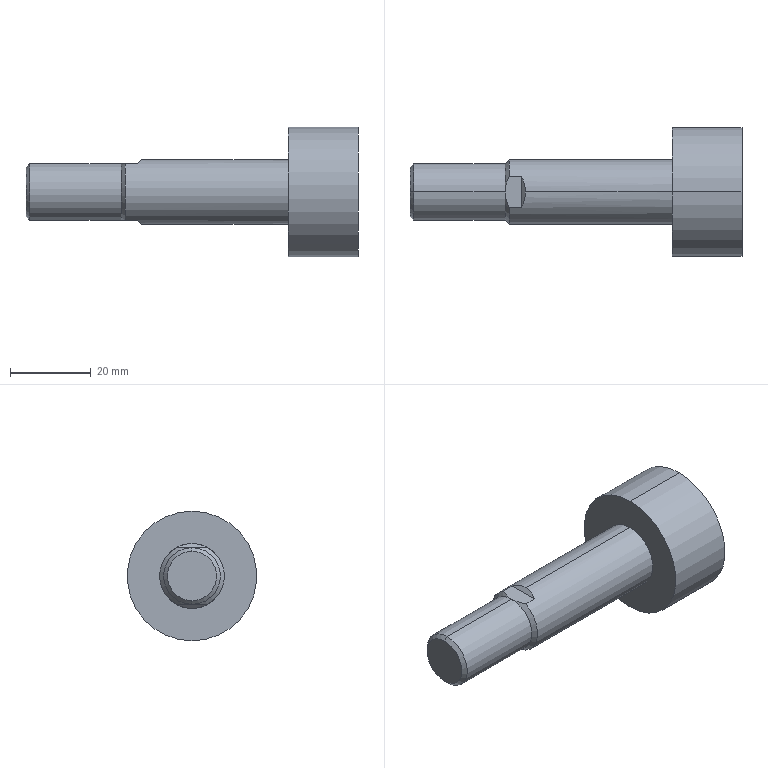Part | SolidWorks | features BaseBody 1 | 1 solid | 17 faces | box 82 x 32 x 32 mm | volume 25673 mm3 | plane 7 | cylinder 6 | cone 4 | commonest cylinder face diameters 14 x2 16 x2 32 x2
STEP:
#1=CARTESIAN_POINT('',(36.3,0.,8.));
#2=VERTEX_POINT('',#1);
#3=CARTESIAN_POINT('',(36.3,0.,-8.));
#4=VERTEX_POINT('',#3);
#5=CARTESIAN_POINT('',(36.3,0.,0.));
#6=DIRECTION('',(1.,0.,0.));
#7=DIRECTION('',(0.,0.,-1.));
#8=AXIS2_PLACEMENT_3D('',#5,#6,#7);
#9=CIRCLE('',#8,8.);
#10=EDGE_CURVE('',#2,#4,#9,.T.);
#11=ORIENTED_EDGE('',*,*,#10,.F.);
#12=CARTESIAN_POINT('',(0.,0.,8.));
#13=VERTEX_POINT('',#12);
#14=CARTESIAN_POINT('',(53.5,0.,8.));
#15=DIRECTION('',(-1.,0.,0.));
#16=VECTOR('',#15,1000.);
#17=LINE('',#14,#16);
#18=EDGE_CURVE('',#2,#13,#17,.T.);
#19=ORIENTED_EDGE('',*,*,#18,.T.);
#20=CARTESIAN_POINT('',(-1.,-3.873,7.));
#21=VERTEX_POINT('',#20);
#22=CARTESIAN_POINT('',(-1.,-3.873,7.));
#23=CARTESIAN_POINT('',(-0.3405,-2.681,7.659));
#24=CARTESIAN_POINT('',(0.,-1.362,8.));
#25=CARTESIAN_POINT('',(0.,0.,8.));
#26=(BOUNDED_CURVE()B_SPLINE_CURVE(3,(#22,#23,#24,#25),.UNSPECIFIED.,.F.,.F.)B_SPLINE_CURVE_WITH_KNOTS((4,4),(5.778,6.283),.UNSPECIFIED.)CURVE()GEOMETRIC_REPRESENTATION_ITEM()RATIONAL_B_SPLINE_CURVE((1.,0.9788,0.9788,1.))REPRESENTATION_ITEM(''));
#27=EDGE_CURVE('',#21,#13,#26,.T.);
#28=ORIENTED_EDGE('',*,*,#27,.F.);
#29=CARTESIAN_POINT('',(-4.,-3.873,7.));
#30=VERTEX_POINT('',#29);
#31=CARTESIAN_POINT('',(53.5,-3.873,7.));
#32=DIRECTION('',(1.,0.,0.));
#33=VECTOR('',#32,1000.);
#34=LINE('',#31,#33);
#35=EDGE_CURVE('',#30,#21,#34,.T.);
#36=ORIENTED_EDGE('',*,*,#35,.F.);
#37=CARTESIAN_POINT('',(-4.,-3.873,-7.));
#38=VERTEX_POINT('',#37);
#39=CARTESIAN_POINT('',(-4.,0.,0.));
#40=DIRECTION('',(1.,0.,0.));
#41=DIRECTION('',(0.,0.,-1.));
#42=AXIS2_PLACEMENT_3D('',#39,#40,#41);
#43=CIRCLE('',#42,8.);
#44=EDGE_CURVE('',#30,#38,#43,.T.);
#45=ORIENTED_EDGE('',*,*,#44,.T.);
#46=CARTESIAN_POINT('',(-1.,-3.873,-7.));
#47=VERTEX_POINT('',#46);
#48=CARTESIAN_POINT('',(53.5,-3.873,-7.));
#49=DIRECTION('',(-1.,0.,0.));
#50=VECTOR('',#49,1000.);
#51=LINE('',#48,#50);
#52=EDGE_CURVE('',#47,#38,#51,.T.);
#53=ORIENTED_EDGE('',*,*,#52,.F.);
#54=CARTESIAN_POINT('',(0.,0.,-8.));
#55=VERTEX_POINT('',#54);
#56=CARTESIAN_POINT('',(0.,0.,-8.));
#57=CARTESIAN_POINT('',(0.,-1.362,-8.));
#58=CARTESIAN_POINT('',(-0.3405,-2.681,-7.659));
#59=CARTESIAN_POINT('',(-1.,-3.873,-7.));
#60=(BOUNDED_CURVE()B_SPLINE_CURVE(3,(#56,#57,#58,#59),.UNSPECIFIED.,.F.,.F.)B_SPLINE_CURVE_WITH_KNOTS((4,4),(0.,0.5054),.UNSPECIFIED.)CURVE()GEOMETRIC_REPRESENTATION_ITEM()RATIONAL_B_SPLINE_CURVE((1.,0.9788,0.9788,1.))REPRESENTATION_ITEM(''));
#61=EDGE_CURVE('',#55,#47,#60,.T.);
#62=ORIENTED_EDGE('',*,*,#61,.F.);
#63=CARTESIAN_POINT('',(53.5,0.,-8.));
#64=DIRECTION('',(-1.,0.,0.));
#65=VECTOR('',#64,1000.);
#66=LINE('',#63,#65);
#67=EDGE_CURVE('',#4,#55,#66,.T.);
#68=ORIENTED_EDGE('',*,*,#67,.F.);
#69=EDGE_LOOP('',(#11,#19,#28,#36,#45,#53,#62,#68));
#70=FACE_OUTER_BOUND('',#69,.T.);
#71=CARTESIAN_POINT('',(53.5,0.,0.));
#72=DIRECTION('',(-1.,0.,0.));
#73=DIRECTION('',(0.,0.,-1.));
#74=AXIS2_PLACEMENT_3D('',#71,#72,#73);
#75=CYLINDRICAL_SURFACE('',#74,8.);
#76=ADVANCED_FACE('',(#70),#75,.T.);
#77=CARTESIAN_POINT('',(-5.,0.,7.));
#78=VERTEX_POINT('',#77);
#79=CARTESIAN_POINT('',(-5.,0.,-7.));
#80=VERTEX_POINT('',#79);
#81=CARTESIAN_POINT('',(-5.,0.,0.));
#82=DIRECTION('',(1.,0.,0.));
#83=DIRECTION('',(0.,0.,-1.));
#84=AXIS2_PLACEMENT_3D('',#81,#82,#83);
#85=CIRCLE('',#84,7.);
#86=EDGE_CURVE('',#78,#80,#85,.T.);
#87=ORIENTED_EDGE('',*,*,#86,.F.);
#88=CARTESIAN_POINT('',(-27.58,0.,7.));
#89=VERTEX_POINT('',#88);
#90=CARTESIAN_POINT('',(0.,0.,7.));
#91=DIRECTION('',(-1.,0.,0.));
#92=VECTOR('',#91,1000.);
#93=LINE('',#90,#92);
#94=EDGE_CURVE('',#78,#89,#93,.T.);
#95=ORIENTED_EDGE('',*,*,#94,.T.);
#96=CARTESIAN_POINT('',(-27.58,0.,-7.));
#97=VERTEX_POINT('',#96);
#98=CARTESIAN_POINT('',(-27.58,0.,0.));
#99=DIRECTION('',(1.,0.,0.));
#100=DIRECTION('',(0.,0.,-1.));
#101=AXIS2_PLACEMENT_3D('',#98,#99,#100);
#102=CIRCLE('',#101,7.);
#103=EDGE_CURVE('',#89,#97,#102,.T.);
#104=ORIENTED_EDGE('',*,*,#103,.T.);
#105=CARTESIAN_POINT('',(0.,0.,-7.));
#106=DIRECTION('',(-1.,0.,0.));
#107=VECTOR('',#106,1000.);
#108=LINE('',#105,#107);
#109=EDGE_CURVE('',#80,#97,#108,.T.);
#110=ORIENTED_EDGE('',*,*,#109,.F.);
#111=EDGE_LOOP('',(#87,#95,#104,#110));
#112=FACE_OUTER_BOUND('',#111,.T.);
#113=CARTESIAN_POINT('',(0.,0.,0.));
#114=DIRECTION('',(-1.,0.,0.));
#115=DIRECTION('',(0.,0.,-1.));
#116=AXIS2_PLACEMENT_3D('',#113,#114,#115);
#117=CYLINDRICAL_SURFACE('',#116,7.);
#118=ADVANCED_FACE('',(#112),#117,.T.);
#119=CARTESIAN_POINT('',(-28.5,0.,-6.08));
#120=VERTEX_POINT('',#119);
#121=CARTESIAN_POINT('',(-28.5,0.,6.08));
#122=VERTEX_POINT('',#121);
#123=CARTESIAN_POINT('',(-28.5,0.,0.));
#124=DIRECTION('',(1.,0.,0.));
#125=DIRECTION('',(0.,0.,-1.));
#126=AXIS2_PLACEMENT_3D('',#123,#124,#125);
#127=CIRCLE('',#126,6.08);
#128=EDGE_CURVE('',#120,#122,#127,.T.);
#129=ORIENTED_EDGE('',*,*,#128,.T.);
#130=CARTESIAN_POINT('',(-28.5,0.,6.08));
#131=DIRECTION('',(0.7071,0.,0.7071));
#132=VECTOR('',#131,1000.);
#133=LINE('',#130,#132);
#134=EDGE_CURVE('',#122,#89,#133,.T.);
#135=ORIENTED_EDGE('',*,*,#134,.T.);
#136=CARTESIAN_POINT('',(-27.58,0.,0.));
#137=DIRECTION('',(1.,0.,0.));
#138=DIRECTION('',(0.,0.,-1.));
#139=AXIS2_PLACEMENT_3D('',#136,#137,#138);
#140=CIRCLE('',#139,7.);
#141=EDGE_CURVE('',#97,#89,#140,.T.);
#142=ORIENTED_EDGE('',*,*,#141,.F.);
#143=CARTESIAN_POINT('',(-28.5,0.,-6.08));
#144=DIRECTION('',(0.7071,0.,-0.7071));
#145=VECTOR('',#144,1000.);
#146=LINE('',#143,#145);
#147=EDGE_CURVE('',#120,#97,#146,.T.);
#148=ORIENTED_EDGE('',*,*,#147,.F.);
#149=EDGE_LOOP('',(#129,#135,#142,#148));
#150=FACE_OUTER_BOUND('',#149,.T.);
#151=CARTESIAN_POINT('',(-28.5,0.,0.));
#152=DIRECTION('',(1.,0.,0.));
#153=DIRECTION('',(0.,0.,-1.));
#154=AXIS2_PLACEMENT_3D('',#151,#152,#153);
#155=CONICAL_SURFACE('',#154,6.08,0.7854);
#156=ADVANCED_FACE('',(#150),#155,.T.);
#157=CARTESIAN_POINT('',(53.5,0.,16.));
#158=VERTEX_POINT('',#157);
#159=CARTESIAN_POINT('',(53.5,0.,-16.));
#160=VERTEX_POINT('',#159);
#161=CARTESIAN_POINT('',(53.5,0.,0.));
#162=DIRECTION('',(1.,0.,0.));
#163=DIRECTION('',(0.,0.,-1.));
#164=AXIS2_PLACEMENT_3D('',#161,#162,#163);
#165=CIRCLE('',#164,16.);
#166=EDGE_CURVE('',#158,#160,#165,.T.);
#167=ORIENTED_EDGE('',*,*,#166,.F.);
#168=CARTESIAN_POINT('',(36.3,0.,16.));
#169=VERTEX_POINT('',#168);
#170=CARTESIAN_POINT('',(53.5,0.,16.));
#171=DIRECTION('',(-1.,0.,0.));
#172=VECTOR('',#171,1000.);
#173=LINE('',#170,#172);
#174=EDGE_CURVE('',#158,#169,#173,.T.);
#175=ORIENTED_EDGE('',*,*,#174,.T.);
#176=CARTESIAN_POINT('',(36.3,0.,-16.));
#177=VERTEX_POINT('',#176);
#178=CARTESIAN_POINT('',(36.3,0.,0.));
#179=DIRECTION('',(1.,0.,0.));
#180=DIRECTION('',(0.,0.,-1.));
#181=AXIS2_PLACEMENT_3D('',#178,#179,#180);
#182=CIRCLE('',#181,16.);
#183=EDGE_CURVE('',#169,#177,#182,.T.);
#184=ORIENTED_EDGE('',*,*,#183,.T.);
#185=CARTESIAN_POINT('',(53.5,0.,-16.));
#186=DIRECTION('',(-1.,0.,0.));
#187=VECTOR('',#186,1000.);
#188=LINE('',#185,#187);
#189=EDGE_CURVE('',#160,#177,#188,.T.);
#190=ORIENTED_EDGE('',*,*,#189,.F.);
#191=EDGE_LOOP('',(#167,#175,#184,#190));
#192=FACE_OUTER_BOUND('',#191,.T.);
#193=CARTESIAN_POINT('',(53.5,0.,0.));
#194=DIRECTION('',(-1.,0.,0.));
#195=DIRECTION('',(0.,0.,-1.));
#196=AXIS2_PLACEMENT_3D('',#193,#194,#195);
#197=CYLINDRICAL_SURFACE('',#196,16.);
#198=ADVANCED_FACE('',(#192),#197,.T.);
#199=CARTESIAN_POINT('',(36.3,0.,0.));
#200=DIRECTION('',(1.,0.,0.));
#201=DIRECTION('',(0.,0.,-1.));
#202=AXIS2_PLACEMENT_3D('',#199,#200,#201);
#203=CIRCLE('',#202,8.);
#204=EDGE_CURVE('',#4,#2,#203,.T.);
#205=ORIENTED_EDGE('',*,*,#204,.T.);
#206=ORIENTED_EDGE('',*,*,#10,.T.);
#207=EDGE_LOOP('',(#205,#206));
#208=FACE_BOUND('',#207,.T.);
#209=CARTESIAN_POINT('',(36.3,0.,0.));
#210=DIRECTION('',(1.,0.,0.));
#211=DIRECTION('',(0.,0.,-1.));
#212=AXIS2_PLACEMENT_3D('',#209,#210,#211);
#213=CIRCLE('',#212,16.);
#214=EDGE_CURVE('',#177,#169,#213,.T.);
#215=ORIENTED_EDGE('',*,*,#214,.F.);
#216=ORIENTED_EDGE('',*,*,#183,.F.);
#217=EDGE_LOOP('',(#215,#216));
#218=FACE_OUTER_BOUND('',#217,.T.);
#219=CARTESIAN_POINT('',(36.3,8.,0.));
#220=DIRECTION('',(1.,0.,0.));
#221=DIRECTION('',(0.,1.,0.));
#222=AXIS2_PLACEMENT_3D('',#219,#220,#221);
#223=PLANE('',#222);
#224=ADVANCED_FACE('',(#208,#218),#223,.F.);
#225=ORIENTED_EDGE('',*,*,#174,.F.);
#226=CARTESIAN_POINT('',(53.5,0.,0.));
#227=DIRECTION('',(1.,0.,0.));
#228=DIRECTION('',(0.,0.,-1.));
#229=AXIS2_PLACEMENT_3D('',#226,#227,#228);
#230=CIRCLE('',#229,16.);
#231=EDGE_CURVE('',#160,#158,#230,.T.);
#232=ORIENTED_EDGE('',*,*,#231,.F.);
#233=ORIENTED_EDGE('',*,*,#189,.T.);
#234=ORIENTED_EDGE('',*,*,#214,.T.);
#235=EDGE_LOOP('',(#225,#232,#233,#234));
#236=FACE_OUTER_BOUND('',#235,.T.);
#237=CARTESIAN_POINT('',(53.5,0.,0.));
#238=DIRECTION('',(-1.,0.,0.));
#239=DIRECTION('',(0.,0.,-1.));
#240=AXIS2_PLACEMENT_3D('',#237,#238,#239);
#241=CYLINDRICAL_SURFACE('',#240,16.);
#242=ADVANCED_FACE('',(#236),#241,.T.);
#243=ORIENTED_EDGE('',*,*,#231,.T.);
#244=ORIENTED_EDGE('',*,*,#166,.T.);
#245=EDGE_LOOP('',(#243,#244));
#246=FACE_OUTER_BOUND('',#245,.T.);
#247=CARTESIAN_POINT('',(53.5,16.,0.));
#248=DIRECTION('',(-1.,0.,0.));
#249=DIRECTION('',(0.,0.,1.));
#250=AXIS2_PLACEMENT_3D('',#247,#248,#249);
#251=PLANE('',#250);
#252=ADVANCED_FACE('',(#246),#251,.F.);
#253=ORIENTED_EDGE('',*,*,#128,.F.);
#254=CARTESIAN_POINT('',(-28.5,0.,0.));
#255=DIRECTION('',(1.,0.,0.));
#256=DIRECTION('',(0.,0.,-1.));
#257=AXIS2_PLACEMENT_3D('',#254,#255,#256);
#258=CIRCLE('',#257,6.08);
#259=EDGE_CURVE('',#122,#120,#258,.T.);
#260=ORIENTED_EDGE('',*,*,#259,.F.);
#261=EDGE_LOOP('',(#253,#260));
#262=FACE_OUTER_BOUND('',#261,.T.);
#263=CARTESIAN_POINT('',(-28.5,0.,0.));
#264=DIRECTION('',(1.,0.,0.));
#265=DIRECTION('',(0.,1.,0.));
#266=AXIS2_PLACEMENT_3D('',#263,#264,#265);
#267=PLANE('',#266);
#268=ADVANCED_FACE('',(#262),#267,.F.);
#269=ORIENTED_EDGE('',*,*,#134,.F.);
#270=ORIENTED_EDGE('',*,*,#259,.T.);
#271=ORIENTED_EDGE('',*,*,#147,.T.);
#272=ORIENTED_EDGE('',*,*,#103,.F.);
#273=EDGE_LOOP('',(#269,#270,#271,#272));
#274=FACE_OUTER_BOUND('',#273,.T.);
#275=CARTESIAN_POINT('',(-28.5,0.,0.));
#276=DIRECTION('',(1.,0.,0.));
#277=DIRECTION('',(0.,0.,-1.));
#278=AXIS2_PLACEMENT_3D('',#275,#276,#277);
#279=CONICAL_SURFACE('',#278,6.08,0.7854);
#280=ADVANCED_FACE('',(#274),#279,.T.);
#281=ORIENTED_EDGE('',*,*,#94,.F.);
#282=CARTESIAN_POINT('',(-5.,0.,0.));
#283=DIRECTION('',(1.,0.,0.));
#284=DIRECTION('',(0.,0.,-1.));
#285=AXIS2_PLACEMENT_3D('',#282,#283,#284);
#286=CIRCLE('',#285,7.);
#287=EDGE_CURVE('',#80,#78,#286,.T.);
#288=ORIENTED_EDGE('',*,*,#287,.F.);
#289=ORIENTED_EDGE('',*,*,#109,.T.);
#290=ORIENTED_EDGE('',*,*,#141,.T.);
#291=EDGE_LOOP('',(#281,#288,#289,#290));
#292=FACE_OUTER_BOUND('',#291,.T.);
#293=CARTESIAN_POINT('',(0.,0.,0.));
#294=DIRECTION('',(-1.,0.,0.));
#295=DIRECTION('',(0.,0.,-1.));
#296=AXIS2_PLACEMENT_3D('',#293,#294,#295);
#297=CYLINDRICAL_SURFACE('',#296,7.);
#298=ADVANCED_FACE('',(#292),#297,.T.);
#299=ORIENTED_EDGE('',*,*,#27,.T.);
#300=CARTESIAN_POINT('',(-1.,3.873,7.));
#301=VERTEX_POINT('',#300);
#302=CARTESIAN_POINT('',(0.,0.,8.));
#303=CARTESIAN_POINT('',(0.,1.362,8.));
#304=CARTESIAN_POINT('',(-0.3405,2.681,7.659));
#305=CARTESIAN_POINT('',(-1.,3.873,7.));
#306=(BOUNDED_CURVE()B_SPLINE_CURVE(3,(#302,#303,#304,#305),.UNSPECIFIED.,.F.,.F.)B_SPLINE_CURVE_WITH_KNOTS((4,4),(0.,0.5054),.UNSPECIFIED.)CURVE()GEOMETRIC_REPRESENTATION_ITEM()RATIONAL_B_SPLINE_CURVE((1.,0.9788,0.9788,1.))REPRESENTATION_ITEM(''));
#307=EDGE_CURVE('',#13,#301,#306,.T.);
#308=ORIENTED_EDGE('',*,*,#307,.T.);
#309=CARTESIAN_POINT('',(-1.,14.,7.));
#310=DIRECTION('',(0.,-1.,0.));
#311=VECTOR('',#310,1000.);
#312=LINE('',#309,#311);
#313=EDGE_CURVE('',#301,#21,#312,.T.);
#314=ORIENTED_EDGE('',*,*,#313,.T.);
#315=EDGE_LOOP('',(#299,#308,#314));
#316=FACE_OUTER_BOUND('',#315,.T.);
#317=CARTESIAN_POINT('',(19.,14.,27.));
#318=DIRECTION('',(-0.7071,0.,0.7071));
#319=DIRECTION('',(0.,1.,0.));
#320=AXIS2_PLACEMENT_3D('',#317,#318,#319);
#321=PLANE('',#320);
#322=ADVANCED_FACE('',(#316),#321,.T.);
#323=CARTESIAN_POINT('',(-4.,3.873,-7.));
#324=VERTEX_POINT('',#323);
#325=CARTESIAN_POINT('',(-5.,0.,-7.));
#326=CARTESIAN_POINT('',(-5.,0.3255,-7.));
#327=CARTESIAN_POINT('',(-4.965,0.8186,-7.));
#328=CARTESIAN_POINT('',(-4.864,1.403,-7.));
#329=CARTESIAN_POINT('',(-4.798,1.697,-7.));
#330=CARTESIAN_POINT('',(-4.761,1.844,-7.));
#331=CARTESIAN_POINT('',(-4.742,1.918,-7.));
#332=CARTESIAN_POINT('',(-4.733,1.95,-7.));
#333=CARTESIAN_POINT('',(-4.728,1.971,-7.));
#334=CARTESIAN_POINT('',(-4.725,1.983,-7.));
#335=CARTESIAN_POINT('',(-4.559,2.589,-7.));
#336=CARTESIAN_POINT('',(-4.318,3.216,-7.));
#337=CARTESIAN_POINT('',(-4.,3.873,-7.));
#338=B_SPLINE_CURVE_WITH_KNOTS('',3,(#325,#326,#327,#328,#329,#330,#331,#332,#333,#334,#335,#336,#337),.UNSPECIFIED.,.F.,.F.,(4,1,1,1,1,1,2,2,4),(0.,0.25,0.375,0.4375,0.4687,0.4844,0.4922,0.5,1.),.UNSPECIFIED.);
#339=EDGE_CURVE('',#80,#324,#338,.T.);
#340=ORIENTED_EDGE('',*,*,#339,.F.);
#341=ORIENTED_EDGE('',*,*,#287,.T.);
#342=CARTESIAN_POINT('',(-4.,3.873,7.));
#343=VERTEX_POINT('',#342);
#344=CARTESIAN_POINT('',(-4.,3.873,7.));
#345=CARTESIAN_POINT('',(-4.159,3.545,7.));
#346=CARTESIAN_POINT('',(-4.368,3.064,7.));
#347=CARTESIAN_POINT('',(-4.562,2.521,7.));
#348=CARTESIAN_POINT('',(-4.646,2.255,7.));
#349=CARTESIAN_POINT('',(-4.685,2.123,7.));
#350=CARTESIAN_POINT('',(-4.704,2.058,7.));
#351=CARTESIAN_POINT('',(-4.712,2.03,7.));
#352=CARTESIAN_POINT('',(-4.717,2.011,7.));
#353=CARTESIAN_POINT('',(-4.719,2.003,7.));
#354=CARTESIAN_POINT('',(-4.907,1.315,7.));
#355=CARTESIAN_POINT('',(-5.,0.6513,7.));
#356=CARTESIAN_POINT('',(-5.,0.,7.));
#357=B_SPLINE_CURVE_WITH_KNOTS('',3,(#344,#345,#346,#347,#348,#349,#350,#351,#352,#353,#354,#355,#356),.UNSPECIFIED.,.F.,.F.,(4,1,1,1,1,1,2,2,4),(0.,0.25,0.375,0.4375,0.4688,0.4844,0.4922,0.5,1.),.UNSPECIFIED.);
#358=EDGE_CURVE('',#343,#78,#357,.T.);
#359=ORIENTED_EDGE('',*,*,#358,.F.);
#360=CARTESIAN_POINT('',(-4.,0.,0.));
#361=DIRECTION('',(1.,0.,0.));
#362=DIRECTION('',(0.,0.,-1.));
#363=AXIS2_PLACEMENT_3D('',#360,#361,#362);
#364=CIRCLE('',#363,8.);
#365=EDGE_CURVE('',#324,#343,#364,.T.);
#366=ORIENTED_EDGE('',*,*,#365,.F.);
#367=EDGE_LOOP('',(#340,#341,#359,#366));
#368=FACE_OUTER_BOUND('',#367,.T.);
#369=CARTESIAN_POINT('',(-5.,0.,0.));
#370=DIRECTION('',(1.,0.,0.));
#371=DIRECTION('',(0.,0.,-1.));
#372=AXIS2_PLACEMENT_3D('',#369,#370,#371);
#373=CONICAL_SURFACE('',#372,7.,0.7854);
#374=ADVANCED_FACE('',(#368),#373,.T.);
#375=CARTESIAN_POINT('',(-5.,0.,7.));
#376=CARTESIAN_POINT('',(-5.,-0.3269,7.));
#377=CARTESIAN_POINT('',(-4.965,-0.8222,7.));
#378=CARTESIAN_POINT('',(-4.863,-1.409,7.));
#379=CARTESIAN_POINT('',(-4.796,-1.704,7.));
#380=CARTESIAN_POINT('',(-4.759,-1.852,7.));
#381=CARTESIAN_POINT('',(-4.74,-1.927,7.));
#382=CARTESIAN_POINT('',(-4.731,-1.959,7.));
#383=CARTESIAN_POINT('',(-4.725,-1.98,7.));
#384=CARTESIAN_POINT('',(-4.722,-1.992,7.));
#385=CARTESIAN_POINT('',(-4.556,-2.595,7.));
#386=CARTESIAN_POINT('',(-4.316,-3.219,7.));
#387=CARTESIAN_POINT('',(-4.,-3.873,7.));
#388=B_SPLINE_CURVE_WITH_KNOTS('',3,(#375,#376,#377,#378,#379,#380,#381,#382,#383,#384,#385,#386,#387),.UNSPECIFIED.,.F.,.F.,(4,1,1,1,1,1,2,2,4),(0.,0.25,0.375,0.4375,0.4688,0.4844,0.4922,0.5,1.),.UNSPECIFIED.);
#389=EDGE_CURVE('',#78,#30,#388,.T.);
#390=ORIENTED_EDGE('',*,*,#389,.F.);
#391=ORIENTED_EDGE('',*,*,#86,.T.);
#392=CARTESIAN_POINT('',(-4.,-3.873,-7.));
#393=CARTESIAN_POINT('',(-4.158,-3.546,-7.));
#394=CARTESIAN_POINT('',(-4.367,-3.067,-7.));
#395=CARTESIAN_POINT('',(-4.56,-2.528,-7.));
#396=CARTESIAN_POINT('',(-4.644,-2.263,-7.));
#397=CARTESIAN_POINT('',(-4.683,-2.132,-7.));
#398=CARTESIAN_POINT('',(-4.701,-2.066,-7.));
#399=CARTESIAN_POINT('',(-4.709,-2.038,-7.));
#400=CARTESIAN_POINT('',(-4.714,-2.02,-7.));
#401=CARTESIAN_POINT('',(-4.717,-2.012,-7.));
#402=CARTESIAN_POINT('',(-4.907,-1.321,-7.));
#403=CARTESIAN_POINT('',(-5.,-0.6541,-7.));
#404=CARTESIAN_POINT('',(-5.,0.,-7.));
#405=B_SPLINE_CURVE_WITH_KNOTS('',3,(#392,#393,#394,#395,#396,#397,#398,#399,#400,#401,#402,#403,#404),.UNSPECIFIED.,.F.,.F.,(4,1,1,1,1,1,2,2,4),(0.,0.25,0.375,0.4375,0.4687,0.4844,0.4922,0.5,1.),.UNSPECIFIED.);
#406=EDGE_CURVE('',#38,#80,#405,.T.);
#407=ORIENTED_EDGE('',*,*,#406,.F.);
#408=ORIENTED_EDGE('',*,*,#44,.F.);
#409=EDGE_LOOP('',(#390,#391,#407,#408));
#410=FACE_OUTER_BOUND('',#409,.T.);
#411=CARTESIAN_POINT('',(-5.,0.,0.));
#412=DIRECTION('',(1.,0.,0.));
#413=DIRECTION('',(0.,0.,-1.));
#414=AXIS2_PLACEMENT_3D('',#411,#412,#413);
#415=CONICAL_SURFACE('',#414,7.,0.7854);
#416=ADVANCED_FACE('',(#410),#415,.T.);
#417=ORIENTED_EDGE('',*,*,#35,.T.);
#418=ORIENTED_EDGE('',*,*,#313,.F.);
#419=CARTESIAN_POINT('',(53.5,3.873,7.));
#420=DIRECTION('',(-1.,0.,0.));
#421=VECTOR('',#420,1000.);
#422=LINE('',#419,#421);
#423=EDGE_CURVE('',#301,#343,#422,.T.);
#424=ORIENTED_EDGE('',*,*,#423,.T.);
#425=ORIENTED_EDGE('',*,*,#358,.T.);
#426=ORIENTED_EDGE('',*,*,#389,.T.);
#427=EDGE_LOOP('',(#417,#418,#424,#425,#426));
#428=FACE_OUTER_BOUND('',#427,.T.);
#429=CARTESIAN_POINT('',(-1.,14.,7.));
#430=DIRECTION('',(0.,0.,1.));
#431=DIRECTION('',(1.,0.,0.));
#432=AXIS2_PLACEMENT_3D('',#429,#430,#431);
#433=PLANE('',#432);
#434=ADVANCED_FACE('',(#428),#433,.T.);
#435=CARTESIAN_POINT('',(-1.,3.873,-7.));
#436=VERTEX_POINT('',#435);
#437=CARTESIAN_POINT('',(-1.,3.873,-7.));
#438=CARTESIAN_POINT('',(-0.3405,2.681,-7.659));
#439=CARTESIAN_POINT('',(0.,1.362,-8.));
#440=CARTESIAN_POINT('',(0.,0.,-8.));
#441=(BOUNDED_CURVE()B_SPLINE_CURVE(3,(#437,#438,#439,#440),.UNSPECIFIED.,.F.,.F.)B_SPLINE_CURVE_WITH_KNOTS((4,4),(5.778,6.283),.UNSPECIFIED.)CURVE()GEOMETRIC_REPRESENTATION_ITEM()RATIONAL_B_SPLINE_CURVE((1.,0.9788,0.9788,1.))REPRESENTATION_ITEM(''));
#442=EDGE_CURVE('',#436,#55,#441,.T.);
#443=ORIENTED_EDGE('',*,*,#442,.T.);
#444=ORIENTED_EDGE('',*,*,#61,.T.);
#445=CARTESIAN_POINT('',(-1.,14.,-7.));
#446=DIRECTION('',(0.,-1.,0.));
#447=VECTOR('',#446,1000.);
#448=LINE('',#445,#447);
#449=EDGE_CURVE('',#436,#47,#448,.T.);
#450=ORIENTED_EDGE('',*,*,#449,.F.);
#451=EDGE_LOOP('',(#443,#444,#450));
#452=FACE_OUTER_BOUND('',#451,.T.);
#453=CARTESIAN_POINT('',(-1.,14.,-7.));
#454=DIRECTION('',(-0.7071,0.,-0.7071));
#455=DIRECTION('',(-0.7071,0.,0.7071));
#456=AXIS2_PLACEMENT_3D('',#453,#454,#455);
#457=PLANE('',#456);
#458=ADVANCED_FACE('',(#452),#457,.T.);
#459=CARTESIAN_POINT('',(53.5,3.873,-7.));
#460=DIRECTION('',(1.,0.,0.));
#461=VECTOR('',#460,1000.);
#462=LINE('',#459,#461);
#463=EDGE_CURVE('',#324,#436,#462,.T.);
#464=ORIENTED_EDGE('',*,*,#463,.T.);
#465=ORIENTED_EDGE('',*,*,#449,.T.);
#466=ORIENTED_EDGE('',*,*,#52,.T.);
#467=ORIENTED_EDGE('',*,*,#406,.T.);
#468=ORIENTED_EDGE('',*,*,#339,.T.);
#469=EDGE_LOOP('',(#464,#465,#466,#467,#468));
#470=FACE_OUTER_BOUND('',#469,.T.);
#471=CARTESIAN_POINT('',(-5.,14.,-7.));
#472=DIRECTION('',(0.,0.,-1.));
#473=DIRECTION('',(0.,-1.,0.));
#474=AXIS2_PLACEMENT_3D('',#471,#472,#473);
#475=PLANE('',#474);
#476=ADVANCED_FACE('',(#470),#475,.T.);
#477=ORIENTED_EDGE('',*,*,#18,.F.);
#478=ORIENTED_EDGE('',*,*,#204,.F.);
#479=ORIENTED_EDGE('',*,*,#67,.T.);
#480=ORIENTED_EDGE('',*,*,#442,.F.);
#481=ORIENTED_EDGE('',*,*,#463,.F.);
#482=ORIENTED_EDGE('',*,*,#365,.T.);
#483=ORIENTED_EDGE('',*,*,#423,.F.);
#484=ORIENTED_EDGE('',*,*,#307,.F.);
#485=EDGE_LOOP('',(#477,#478,#479,#480,#481,#482,#483,#484));
#486=FACE_OUTER_BOUND('',#485,.T.);
#487=CARTESIAN_POINT('',(53.5,0.,0.));
#488=DIRECTION('',(-1.,0.,0.));
#489=DIRECTION('',(0.,0.,-1.));
#490=AXIS2_PLACEMENT_3D('',#487,#488,#489);
#491=CYLINDRICAL_SURFACE('',#490,8.);
#492=ADVANCED_FACE('',(#486),#491,.T.);
#493=CLOSED_SHELL('',(#76,#118,#156,#198,#224,#242,#252,#268,#280,#298,#322,#374,#416,#434,#458,#476,#492));
#494=MANIFOLD_SOLID_BREP('',#493);
#495=CARTESIAN_POINT('',(0.,0.,0.));
#496=DIRECTION('',(0.,0.,1.));
#497=DIRECTION('',(1.,0.,0.));
#498=AXIS2_PLACEMENT_3D('',#495,#496,#497);
#499=(LENGTH_UNIT()NAMED_UNIT(*)SI_UNIT(.MILLI.,.METRE.));
#500=UNCERTAINTY_MEASURE_WITH_UNIT(LENGTH_MEASURE(0.00001),#499,'','');
#501=(NAMED_UNIT(*)PLANE_ANGLE_UNIT()SI_UNIT($,.RADIAN.));
#502=(NAMED_UNIT(*)SI_UNIT($,.STERADIAN.)SOLID_ANGLE_UNIT());
#503=(GEOMETRIC_REPRESENTATION_CONTEXT(3)GLOBAL_UNCERTAINTY_ASSIGNED_CONTEXT((#500))GLOBAL_UNIT_ASSIGNED_CONTEXT((#499,#501,#502))REPRESENTATION_CONTEXT('',''));
#504=ADVANCED_BREP_SHAPE_REPRESENTATION('',(#494,#498),#503);